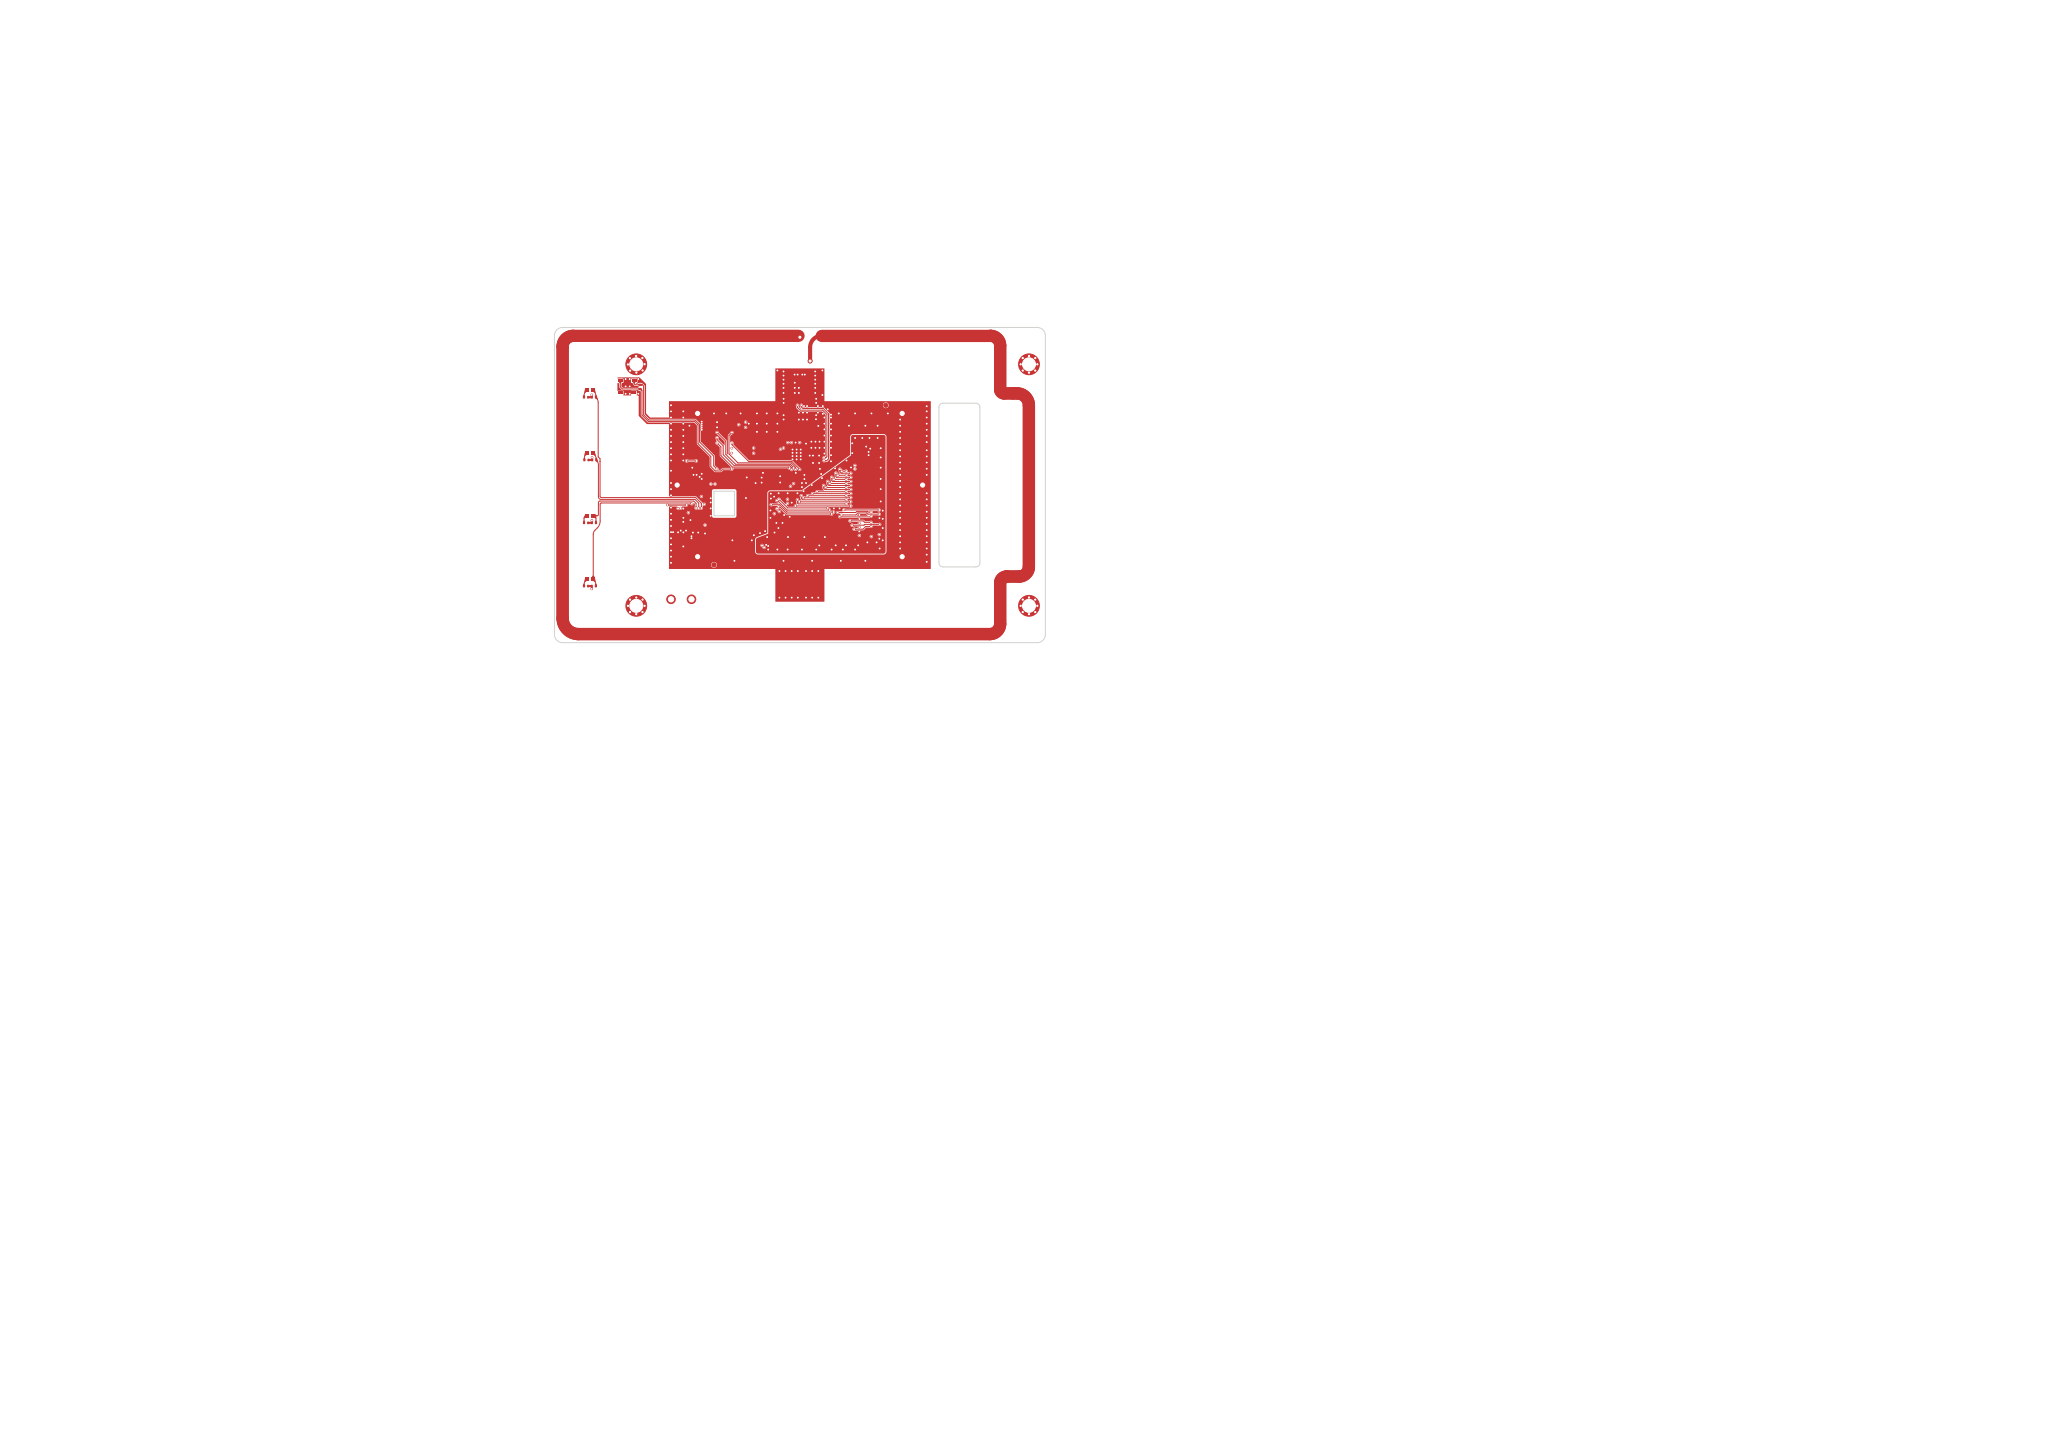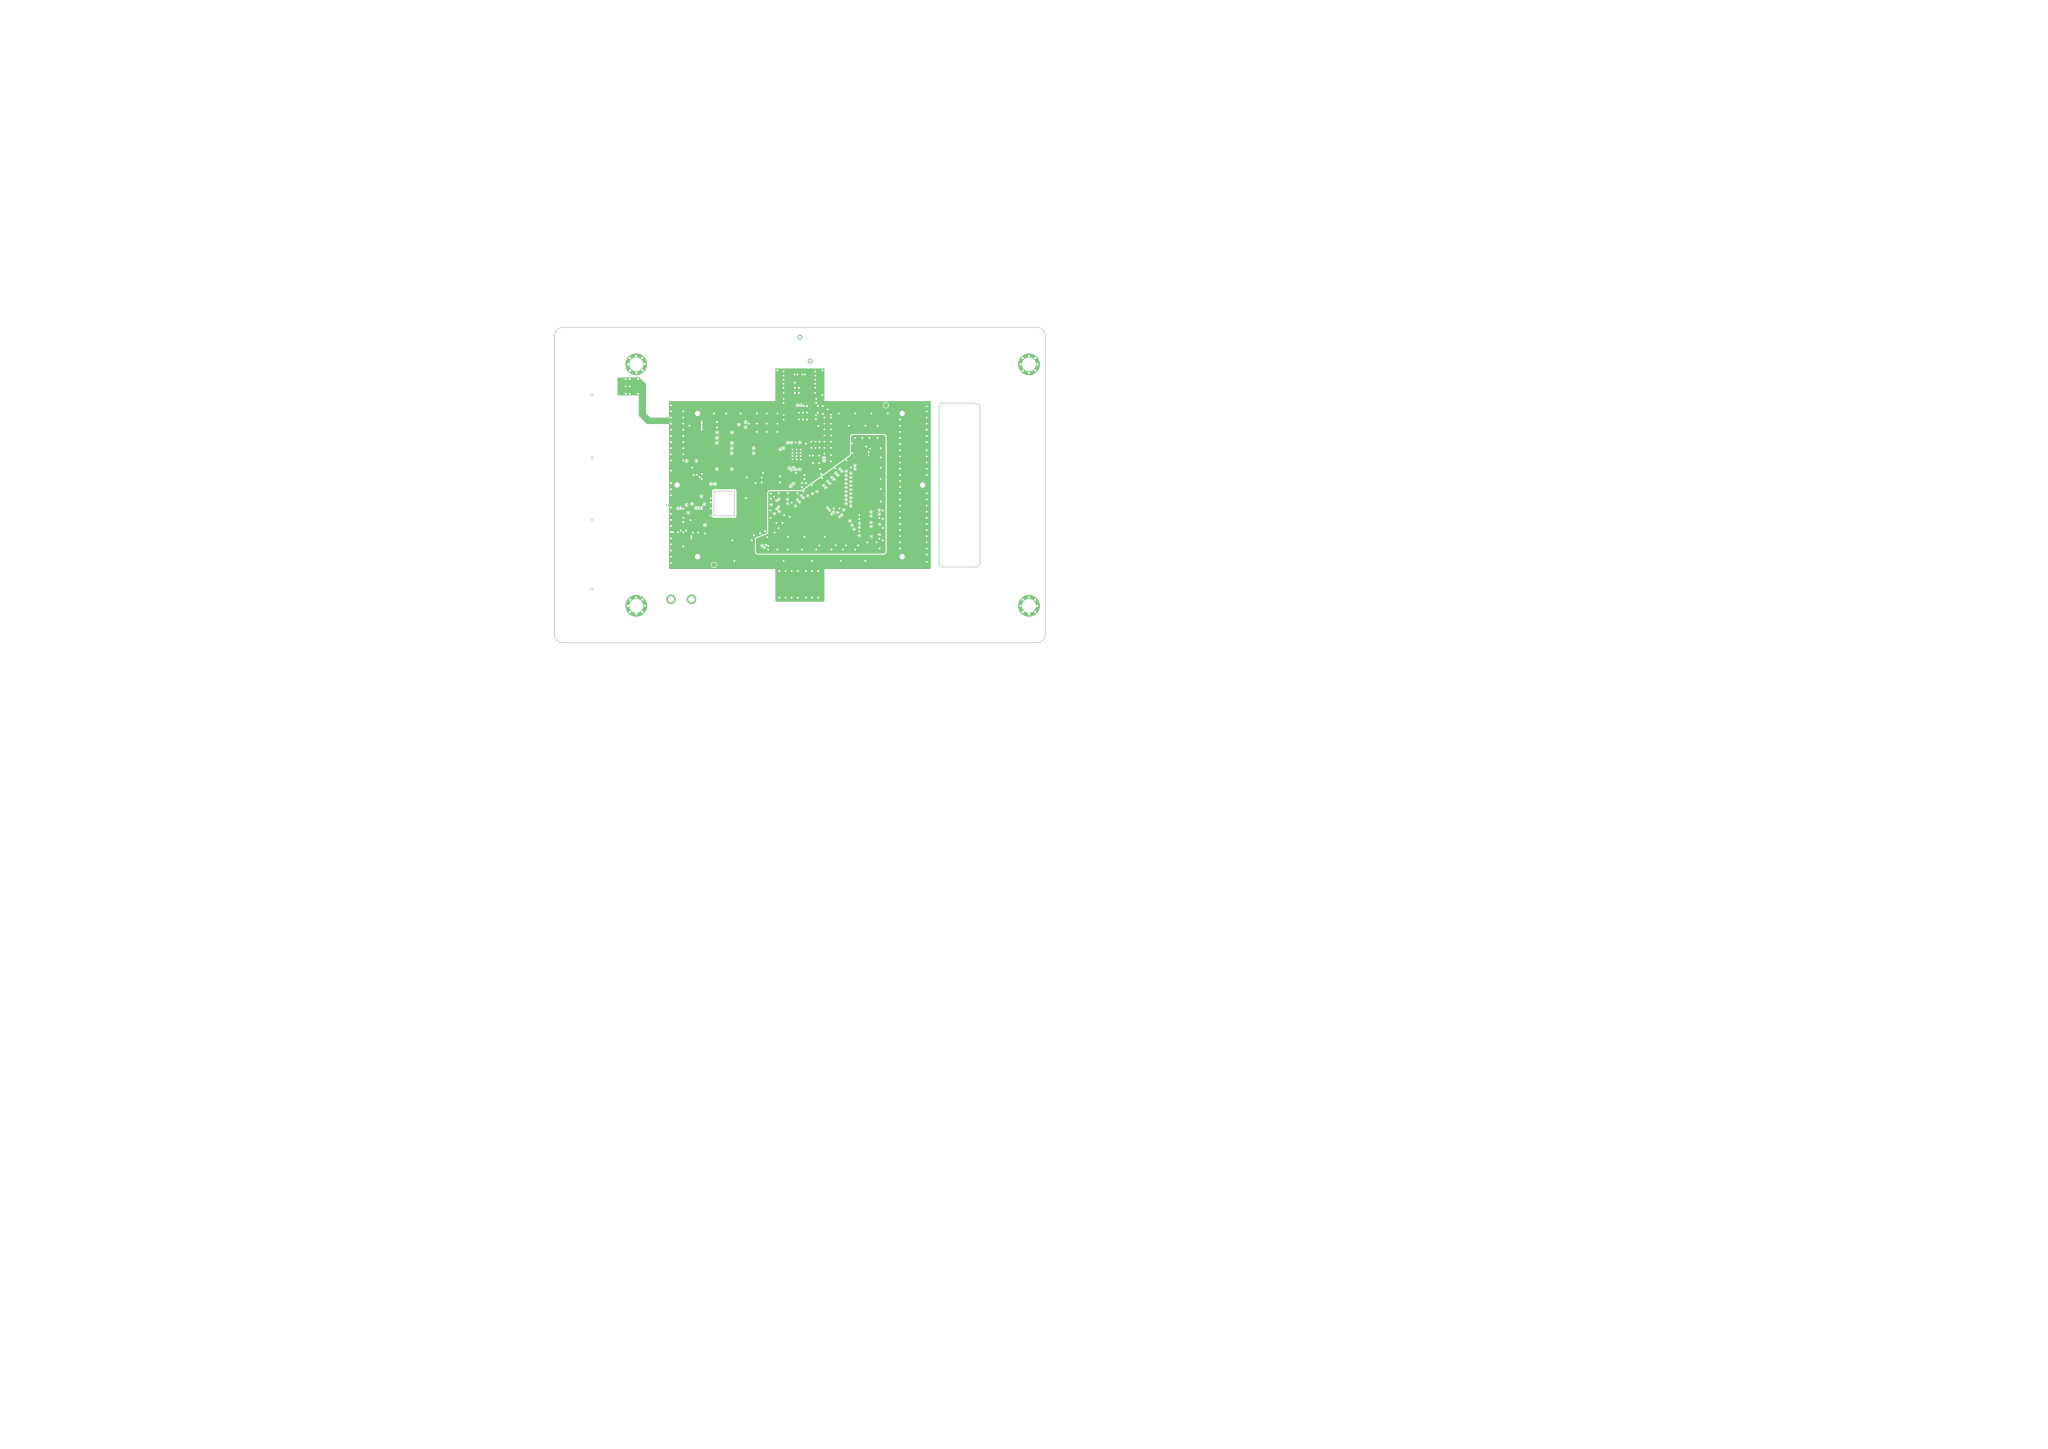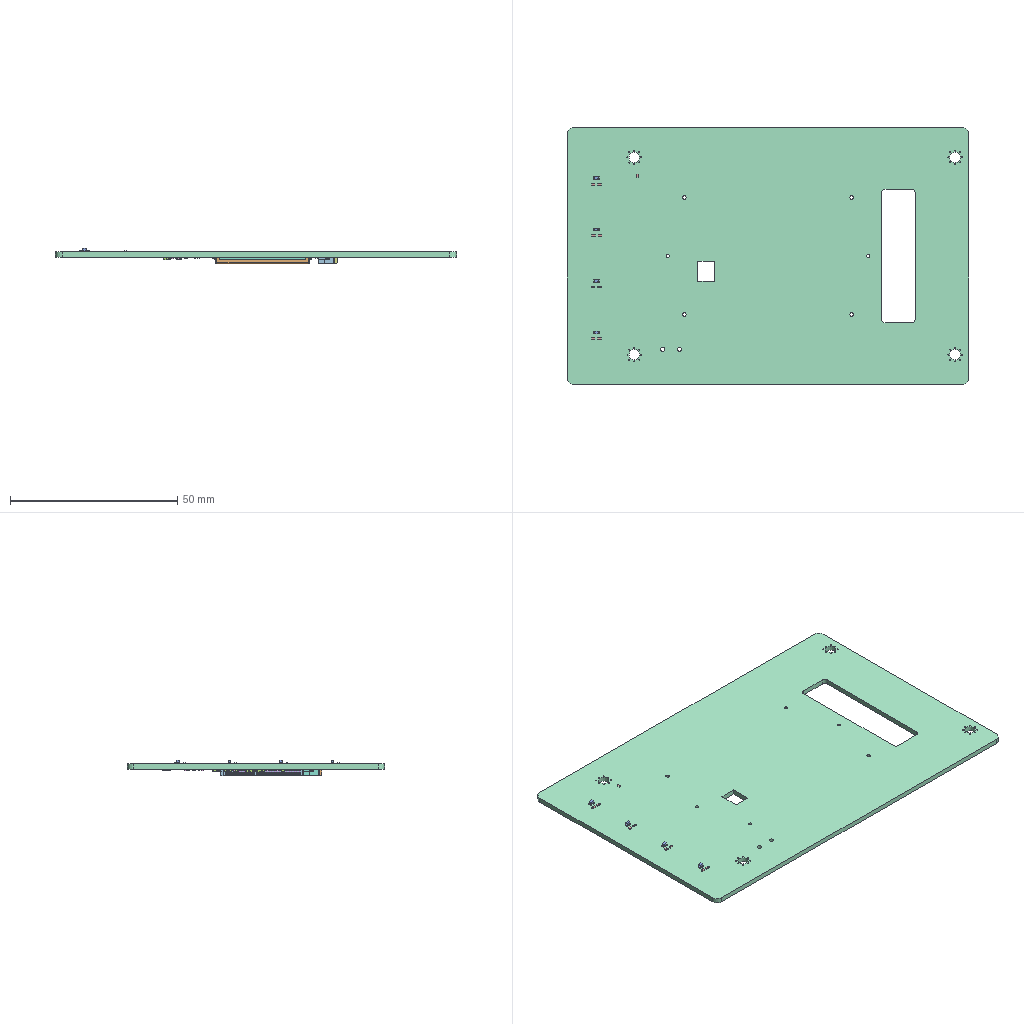Circuit board layout | KiCad | box 120 x 77 x 4.8 mm
Layer stack:
layer,type,thickness_mm,material,epsilon_r
F.Cu,copper (signal),,,
In1.Cu,copper (power),,,
In2.Cu,copper (power),,,
B.Cu,copper (signal),,,
# board thickness,1.6,,,
Part placement:
Ref,Val,Package,PosX,PosY,Rot,Side
C1,CAP-SM,C_0402_1005Metric,126.383,-98.329,180,bottom
C2,CAP-SM,C_0603_1608Metric,126.383,-97.079,180,bottom
C3,CAP-SM,C_0603_1608Metric,149.083,-103.879,-90,bottom
C4,CAP-SM,C_0402_1005Metric,148.783,-101.804,0,bottom
C5,CAP-SM,C_0603_1608Metric,143.552,-92.487,90,bottom
C6,CAP-SM,C_0402_1005Metric,145.822,-92.705,-90,bottom
C7,CAP-SM,C_0402_1005Metric,152.083,-84.179,90,bottom
C8,CAP,C_0402_1005Metric,151.133,-84.179,90,bottom
C9,CAP-SM,C_0402_1005Metric,126.708,-105.854,-90,bottom
C10,CAP-SM,C_0603_1608Metric,125.433,-105.854,-90,bottom
C11,CAP-SM,C_0603_1608Metric,144.883,-98.829,90,bottom
C12,CAP-SM,C_0402_1005Metric,146.083,-98.829,-90,bottom
C13,CAP-SM,C_0603_1608Metric,156.383,-102.079,0,bottom
C14,CAP-SM,C_0402_1005Metric,156.383,-100.829,180,bottom
C15,CAP-SM,C_0402_1005Metric,153.033,-84.179,90,bottom
C16,CAP,C_0402_1005Metric,153.983,-84.179,90,bottom
C17,CAP-SM,C_0603_1608Metric,144.863,-95.82,-90,bottom
C18,CAP-SM,C_0603_1608Metric,143.313,-95.82,-90,bottom
C19,CAP-SM,C_0402_1005Metric,146.113,-95.529,90,bottom
C20,CAP-SM,C_0402_1005Metric,127.708,-105.854,-90,bottom
C21,CAP-SM,C_0402_1005Metric,131.803,-105.479,0,bottom
C22,CAP-SM,C_0402_1005Metric,150.683,-101.804,0,bottom
C23,CAP-SM,C_0402_1005Metric,155.663,-88.704,0,bottom
C24,CAP-SM,C_0402_1005Metric,155.663,-87.704,0,bottom
C25,CAP-SM,C_0402_1005Metric,156.183,-86.204,90,bottom
C26,CAP-SM,C_0402_1005Metric,155.208,-86.204,90,bottom
C27,CAP-SM,C_0402_1005Metric,155.663,-83.704,0,bottom
C28,CAP-SM,C_0402_1005Metric,155.663,-84.704,0,bottom
C29,CAP-SM,C_0402_1005Metric,153.283,-78.879,180,bottom
C30,CAP-SM,C_0402_1005Metric,149.703,-88.754,0,bottom
C31,CAP-SM,C_0402_1005Metric,149.703,-87.704,0,bottom
C32,CAP-SM,C_0402_1005Metric,149.203,-86.204,90,bottom
C33,CAP-SM,C_0402_1005Metric,149.703,-83.704,0,bottom
C34,CAP-SM,C_0402_1005Metric,149.703,-84.704,0,bottom
C35,TRIM_CAP,TSC3S,151.883,-81.279,90,bottom
C36,CAP-SM,C_0402_1005Metric,150.183,-86.204,90,bottom
C37,CAP-SM,C_0402_1005Metric,146.883,-101.804,0,bottom
C38,CAP-SM,C_0402_1005Metric,144.683,-101.804,180,bottom
C43,CAP-SM,C_0603_1608Metric,126.383,-103.279,0,bottom
C44,CAP-SM,C_0402_1005Metric,148.621,-111.245,0,bottom
C45,CAP-SM,C_0603_1608Metric,147.208,-112.804,0,bottom
C46,CAP-SM,C_0402_1005Metric,129.133,-108.179,0,bottom
C47,CAP-SM,C_0603_1608Metric,129.708,-106.929,0,bottom
C54,CAP-SM,C_0402_1005Metric,134.433,-114.779,90,bottom
C142,CAP-SM,C_0402_1005Metric,129.495,-115.517,90,bottom
J1,3220-20-0300-00,3220-20-0300-00,135.983,-95.129,-90,bottom
J2,LCM-50PIN-ANT,LCD-50P-ANT,154.683,-118.549,180,bottom
J3,62684-452100ALF,LCD-45P-0.5MM,171.083,-106.879,-90,bottom
J4,FH34SRJ-6S-0.5SH(50),LCD-6P-0.5,146.395,-109.329,90,bottom
L1,FBMH1608HM102,FBMH1608HM102,147.183,-95.779,-90,bottom
L2,FBMH1608HM102,FBMH1608HM102,129.458,-105.454,0,bottom
L3,IND-SMD,INDC1608X90N,150.383,-103.679,-90,bottom
L4,1206CS-221XGLC,1206CS-221XGLC,154.933,-91.479,45,bottom
L5,1206CS-221XGLC,1206CS-221XGLC,150.408,-91.479,135,bottom
L9,RADIAL_IND,13R332C,123.683,-132.679,180,bottom
Q1,ZXM61N02FTA,ZXM61N02F,167.633,-97.729,0,bottom
Q3,ZXM61N02FTA,ZXM61N02F,131.933,-114.779,-90,bottom
R1,R1206,R_0805_2012Metric,155.183,-77.979,90,bottom
R2,R1206,R_0805_2012Metric,150.183,-77.979,90,bottom
R4,RES-SM,R_0402_1005Metric,129.183,-104.204,180,bottom
R5,RES-SM,R_0402_1005Metric,128.783,-100.079,90,bottom
R7,RES-SM,R_0402_1005Metric,140.303,-95.709,180,bottom
R8,RES-SM,R_0402_1005Metric,140.303,-97.009,180,bottom
R9,RES-SM,R_0402_1005Metric,148.615,-108.254,180,bottom
R10,RES-SM,R_0402_1005Metric,148.615,-110.254,180,bottom
R11,RES-SM,R_0402_1005Metric,148.615,-109.254,180,bottom
R12,RES-SM,R_0402_1005Metric,168.293,-117.079,0,bottom
R13,RES-SM,R_0402_1005Metric,168.293,-114.079,180,bottom
R14,RES-SM,R_0402_1005Metric,168.293,-113.079,0,bottom
R15,RES-SM,R_0402_1005Metric,168.293,-115.079,0,bottom
R16,RES-SM,R_0402_1005Metric,168.293,-116.079,0,bottom
R17,RES-SM,R_0402_1005Metric,168.293,-111.079,0,bottom
R18,RES-SM,R_0402_1005Metric,168.293,-112.079,0,bottom
R19,RES-SM,R_0402_1005Metric,167.633,-95.379,0,bottom
R20,RES-SM,R_0603_1608Metric,167.657,-100.378,0,bottom
R21,RES-SM,R_0402_1005Metric,135.433,-114.779,90,bottom
R22,RES-SM,R_0402_1005Metric,152.683,-77.279,90,bottom
R24,RES-SM,R_0402_1005Metric,129.983,-109.979,90,bottom
R34,RES-SM,R_0402_1005Metric,140.308,-98.304,180,bottom
TH1,THERMAL_40/80,THERMAL_40$2F$80,122.683,-104.779,180,bottom
TH2,THERMAL_40/80,THERMAL_40$2F$80,182.683,-104.779,180,bottom
TH3,THERMAL_40/80,THERMAL_40$2F$80,127.683,-122.279,180,bottom
TH4,THERMAL_40/80,THERMAL_40$2F$80,177.683,-122.279,180,bottom
TH5,THERMAL_40/80,THERMAL_40$2F$80,177.683,-87.279,180,bottom
TH6,THERMAL_40/80,THERMAL_40$2F$80,127.683,-87.279,180,bottom
TP1,TP,TP_SM40,153.383,-93.504,0,bottom
TP2,TP,TP_SM40,151.983,-93.479,0,bottom
U1,ST25R3920_1,ST25R3920,151.883,-97.479,0,bottom
U2,LP38693SD-5.0/NOPB,LP38693SD-5.0$2F$NOPB,126.383,-100.529,180,bottom
U3,PCA9536DGKRG4,DGK8,127.633,-111.379,180,bottom
U5,CAT24C64,TSSOP8,123.883,-114.479,180,bottom
U11,M24SR64-YMC6T/2,UFDFPN8,127.833,-116.379,180,bottom
X1,ABM8-27.120MHZ-D2Y-T,XTAL_3.6X2.8,145.783,-104.154,0,bottom
FM1,FM-40/80,FM-40$2F$80,173.683,-83.279,0,top
FM2,FM-40/80,FM-40$2F$80,131.683,-126.279,0,top
LED1,LED,LED_0603_A,101.384,-127.678,0,top
LED2,LED,LED_0603_A,101.357,-81.484,0,top
LED3,LED,LED_0603_A,101.357,-96.874,0,top
LED4,LED,LED_0603_A,101.374,-112.274,0,top
M1,MT_VIA,MT-200$2F$125_VIA,112.683,-75.279,1,top
M2,MT_VIA,MT-200$2F$125_VIA,112.689,-134.279,0,top
M3,MT_VIA,MT-200$2F$125_VIA,208.683,-75.279,0,top
M4,MT_VIA,MT-200$2F$125_VIA,208.683,-134.279,0,top
R6,RES-SM,R_0402_1005Metric,113.683,-80.789,90,top
R26,RES-SM,R_0402_1005Metric,100.416,-129.454,180,top
R27,RES-SM,R_0402_1005Metric,102.306,-129.454,180,top
R28,RES-SM,R_0402_1005Metric,100.423,-83.33,180,top
R29,RES-SM,R_0402_1005Metric,102.323,-83.33,180,top
R30,RES-SM,R_0402_1005Metric,100.515,-98.654,180,top
R31,RES-SM,R_0402_1005Metric,102.415,-98.654,180,top
R32,RES-SM,R_0402_1005Metric,100.429,-114.011,180,top
R33,RES-SM,R_0402_1005Metric,102.329,-114.011,180,top
S1,ESE13,ESE13,110.483,-80.779,-90,top
Pad and via stacks:
via_type,start_layer,end_layer,diameter_mm,drill_mm,count
through,F.Cu,B.Cu,0.4,0.2,458
through,F.Cu,B.Cu,1,0.5,2
Design rules, without the lines most boards share:
# KiCad design rules of  (from the KiCad project file, unit mm)
max_error = 0.005
min_clearance = 0.0
min_connection = 0.0
min_copper_edge_clearance = 0.5
min_groove_width = 0.0
min_hole_clearance = 0.25
min_hole_to_hole = 0.25
min_microvia_diameter = 0.2
min_microvia_drill = 0.1
min_resolved_spokes = 2
min_silk_clearance = 0.0
min_text_height = 0.8
min_text_thickness = 0.08
min_through_hole_diameter = 0.2
min_track_width = 0.0
min_via_annular_width = 0.1
min_via_diameter = 0.4
solder_mask_to_copper_clearance = 0.0
use_height_for_length_calcs = True
defaults = {"apply_defaults_to_fp_fields": false, "apply_defaults_to_fp_shapes": false, "apply_defaults_to_fp_text": false, "board_outline_line_width": 0.05, "copper_line_width": 0.2, "copper_text_italic": false, "copper_text_size_h": 1.5, "copper_text_size_v": 1.5, "copper_text_thickness": 0.3, "copper_text_upright": false, "courtyard_line_width": 0.05, "dimension_precision": 4, "dimension_units": 3, "dimensions": {"arrow_length": 1270000, "extension_offset": 500000, "keep_text_aligned": true, "suppress_zeroes": true, "text_position": 0, "units_format": 0}, "fab_line_width": 0.1, "fab_text_italic": false, "fab_text_size_h": 1.0, "fab_text_size_v": 1.0, "fab_text_thickness": 0.15, "fab_text_upright": false, "other_line_width": 0.1, "other_text_italic": false, "other_text_size_h": 1.0, "other_text_size_v": 1.0, "other_text_thickness": 0.15, "other_text_upright": false, "pads": {"drill": 0.0, "height": 1.016, "width": 1.016}, "silk_line_width": 0.1, "silk_text_italic": false, "silk_text_size_h": 1.0, "silk_text_size_v": 1.0, "silk_text_thickness": 0.1, "silk_text_upright": false, "zones": {"min_clearance": 0.0}}
track_widths = [0.0, 0.15, 0.2, 0.3, 0.5, 0.7, 1.0]
via_dimensions = [{"diameter": 0.0, "drill": 0.0}, {"diameter": 0.4, "drill": 0.2}, {"diameter": 0.55, "drill": 0.3}, {"diameter": 1.0, "drill": 0.5}]
diff_pair_dimensions = [{"gap": 0.0, "via_gap": 0.0, "width": 0.0}]
# copper zones (pour): pad connection, clearance mm, minimum width mm, count
Classes set for this board:
# KiCad net classes of  (from the KiCad project file, unit mm)
{"bus_width": 12, "clearance": 0.2, "diff_pair_gap": 0.25, "diff_pair_via_gap": 0.25, "diff_pair_width": 0.2, "line_style": 0, "microvia_diameter": 0.3, "microvia_drill": 0.1, "name": "Default", "pcb_color": "rgba(0, 0, 0, 0.000)", "priority": 2147483647, "schematic_color": "rgba(0, 0, 0, 0.000)", "track_width": 0.2, "via_diameter": 0.6, "via_drill": 0.3, "wire_width": 6}